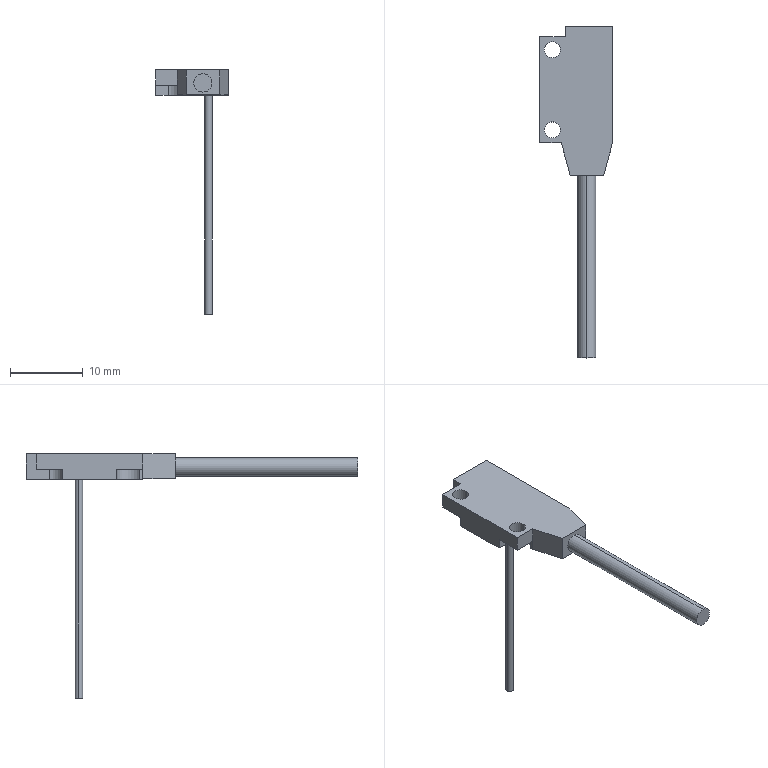Part | SolidWorks | features ICE 3, BaseBody 2 | 1 solid | 43 faces | box 10 x 45.5 x 33.5 mm | volume 726.533 mm3 | plane 31 | cylinder 12 | commonest cylinder face diameters 2.2 x4 1 x2 2 x2 2.5 x2 3.6 x2
STEP:
#1=CARTESIAN_POINT('',(-6.6,4.,21.4));
#2=VERTEX_POINT('',#1);
#3=CARTESIAN_POINT('',(-4.4,4.,21.4));
#4=VERTEX_POINT('',#3);
#5=CARTESIAN_POINT('',(-5.5,4.,21.4));
#6=DIRECTION('',(0.,0.,1.));
#7=DIRECTION('',(1.,0.,0.));
#8=AXIS2_PLACEMENT_3D('',#5,#6,#7);
#9=CIRCLE('',#8,1.1);
#10=EDGE_CURVE('',#2,#4,#9,.T.);
#11=ORIENTED_EDGE('',*,*,#10,.F.);
#12=CARTESIAN_POINT('',(-6.6,4.,23.5));
#13=VERTEX_POINT('',#12);
#14=CARTESIAN_POINT('',(-6.6,4.,20.));
#15=DIRECTION('',(0.,0.,1.));
#16=VECTOR('',#15,1000.);
#17=LINE('',#14,#16);
#18=EDGE_CURVE('',#2,#13,#17,.T.);
#19=ORIENTED_EDGE('',*,*,#18,.T.);
#20=CARTESIAN_POINT('',(-4.4,4.,23.5));
#21=VERTEX_POINT('',#20);
#22=CARTESIAN_POINT('',(-5.5,4.,23.5));
#23=DIRECTION('',(0.,0.,-1.));
#24=DIRECTION('',(1.,0.,0.));
#25=AXIS2_PLACEMENT_3D('',#22,#23,#24);
#26=CIRCLE('',#25,1.1);
#27=EDGE_CURVE('',#21,#13,#26,.T.);
#28=ORIENTED_EDGE('',*,*,#27,.F.);
#29=CARTESIAN_POINT('',(-4.4,4.,20.));
#30=DIRECTION('',(0.,0.,1.));
#31=VECTOR('',#30,1000.);
#32=LINE('',#29,#31);
#33=EDGE_CURVE('',#4,#21,#32,.T.);
#34=ORIENTED_EDGE('',*,*,#33,.F.);
#35=EDGE_LOOP('',(#11,#19,#28,#34));
#36=FACE_OUTER_BOUND('',#35,.T.);
#37=CARTESIAN_POINT('',(-5.5,4.,20.));
#38=DIRECTION('',(0.,0.,1.));
#39=DIRECTION('',(1.,0.,0.));
#40=AXIS2_PLACEMENT_3D('',#37,#38,#39);
#41=CYLINDRICAL_SURFACE('',#40,1.1);
#42=ADVANCED_FACE('',(#36),#41,.F.);
#43=CARTESIAN_POINT('',(-6.6,-7.,21.4));
#44=VERTEX_POINT('',#43);
#45=CARTESIAN_POINT('',(-4.4,-7.,21.4));
#46=VERTEX_POINT('',#45);
#47=CARTESIAN_POINT('',(-5.5,-7.,21.4));
#48=DIRECTION('',(0.,0.,1.));
#49=DIRECTION('',(1.,0.,0.));
#50=AXIS2_PLACEMENT_3D('',#47,#48,#49);
#51=CIRCLE('',#50,1.1);
#52=EDGE_CURVE('',#44,#46,#51,.T.);
#53=ORIENTED_EDGE('',*,*,#52,.F.);
#54=CARTESIAN_POINT('',(-6.6,-7.,23.5));
#55=VERTEX_POINT('',#54);
#56=CARTESIAN_POINT('',(-6.6,-7.,20.));
#57=DIRECTION('',(0.,0.,1.));
#58=VECTOR('',#57,1000.);
#59=LINE('',#56,#58);
#60=EDGE_CURVE('',#44,#55,#59,.T.);
#61=ORIENTED_EDGE('',*,*,#60,.T.);
#62=CARTESIAN_POINT('',(-4.4,-7.,23.5));
#63=VERTEX_POINT('',#62);
#64=CARTESIAN_POINT('',(-5.5,-7.,23.5));
#65=DIRECTION('',(0.,0.,-1.));
#66=DIRECTION('',(1.,0.,0.));
#67=AXIS2_PLACEMENT_3D('',#64,#65,#66);
#68=CIRCLE('',#67,1.1);
#69=EDGE_CURVE('',#63,#55,#68,.T.);
#70=ORIENTED_EDGE('',*,*,#69,.F.);
#71=CARTESIAN_POINT('',(-4.4,-7.,20.));
#72=DIRECTION('',(0.,0.,1.));
#73=VECTOR('',#72,1000.);
#74=LINE('',#71,#73);
#75=EDGE_CURVE('',#46,#63,#74,.T.);
#76=ORIENTED_EDGE('',*,*,#75,.F.);
#77=EDGE_LOOP('',(#53,#61,#70,#76));
#78=FACE_OUTER_BOUND('',#77,.T.);
#79=CARTESIAN_POINT('',(-5.5,-7.,20.));
#80=DIRECTION('',(0.,0.,1.));
#81=DIRECTION('',(1.,0.,0.));
#82=AXIS2_PLACEMENT_3D('',#79,#80,#81);
#83=CYLINDRICAL_SURFACE('',#82,1.1);
#84=ADVANCED_FACE('',(#78),#83,.F.);
#85=CARTESIAN_POINT('',(-0.75,-38.25,22.95));
#86=VERTEX_POINT('',#85);
#87=CARTESIAN_POINT('',(-0.75,-38.25,20.45));
#88=VERTEX_POINT('',#87);
#89=CARTESIAN_POINT('',(-0.75,-38.25,21.7));
#90=DIRECTION('',(0.,1.,0.));
#91=DIRECTION('',(0.,0.,1.));
#92=AXIS2_PLACEMENT_3D('',#89,#90,#91);
#93=CIRCLE('',#92,1.25);
#94=EDGE_CURVE('',#86,#88,#93,.T.);
#95=ORIENTED_EDGE('',*,*,#94,.T.);
#96=CARTESIAN_POINT('',(-0.75,-13.25,20.45));
#97=VERTEX_POINT('',#96);
#98=CARTESIAN_POINT('',(-0.75,-38.25,20.45));
#99=DIRECTION('',(0.,1.,0.));
#100=VECTOR('',#99,1000.);
#101=LINE('',#98,#100);
#102=EDGE_CURVE('',#88,#97,#101,.T.);
#103=ORIENTED_EDGE('',*,*,#102,.T.);
#104=CARTESIAN_POINT('',(-0.75,-13.25,22.95));
#105=VERTEX_POINT('',#104);
#106=CARTESIAN_POINT('',(-0.75,-13.25,21.7));
#107=DIRECTION('',(0.,-1.,0.));
#108=DIRECTION('',(0.,0.,1.));
#109=AXIS2_PLACEMENT_3D('',#106,#107,#108);
#110=CIRCLE('',#109,1.25);
#111=EDGE_CURVE('',#97,#105,#110,.T.);
#112=ORIENTED_EDGE('',*,*,#111,.T.);
#113=CARTESIAN_POINT('',(-0.75,-38.25,22.95));
#114=DIRECTION('',(0.,1.,0.));
#115=VECTOR('',#114,1000.);
#116=LINE('',#113,#115);
#117=EDGE_CURVE('',#86,#105,#116,.T.);
#118=ORIENTED_EDGE('',*,*,#117,.F.);
#119=EDGE_LOOP('',(#95,#103,#112,#118));
#120=FACE_OUTER_BOUND('',#119,.T.);
#121=CARTESIAN_POINT('',(-0.75,-38.25,21.7));
#122=DIRECTION('',(0.,1.,0.));
#123=DIRECTION('',(0.,0.,1.));
#124=AXIS2_PLACEMENT_3D('',#121,#122,#123);
#125=CYLINDRICAL_SURFACE('',#124,1.25);
#126=ADVANCED_FACE('',(#120),#125,.T.);
#127=CARTESIAN_POINT('',(1.,0.,20.1));
#128=VERTEX_POINT('',#127);
#129=CARTESIAN_POINT('',(-1.,0.,20.1));
#130=VERTEX_POINT('',#129);
#131=CARTESIAN_POINT('',(0.,0.,20.1));
#132=DIRECTION('',(0.,0.,-1.));
#133=DIRECTION('',(-1.,0.,0.));
#134=AXIS2_PLACEMENT_3D('',#131,#132,#133);
#135=CIRCLE('',#134,1.);
#136=EDGE_CURVE('',#128,#130,#135,.T.);
#137=ORIENTED_EDGE('',*,*,#136,.F.);
#138=CARTESIAN_POINT('',(1.,0.,20.));
#139=VERTEX_POINT('',#138);
#140=CARTESIAN_POINT('',(1.,0.,20.1));
#141=DIRECTION('',(0.,0.,-1.));
#142=VECTOR('',#141,1000.);
#143=LINE('',#140,#142);
#144=EDGE_CURVE('',#128,#139,#143,.T.);
#145=ORIENTED_EDGE('',*,*,#144,.T.);
#146=CARTESIAN_POINT('',(-1.,0.,20.));
#147=VERTEX_POINT('',#146);
#148=CARTESIAN_POINT('',(0.,0.,20.));
#149=DIRECTION('',(0.,0.,-1.));
#150=DIRECTION('',(-1.,0.,0.));
#151=AXIS2_PLACEMENT_3D('',#148,#149,#150);
#152=CIRCLE('',#151,1.);
#153=EDGE_CURVE('',#139,#147,#152,.T.);
#154=ORIENTED_EDGE('',*,*,#153,.T.);
#155=CARTESIAN_POINT('',(-1.,0.,20.1));
#156=DIRECTION('',(0.,0.,-1.));
#157=VECTOR('',#156,1000.);
#158=LINE('',#155,#157);
#159=EDGE_CURVE('',#130,#147,#158,.T.);
#160=ORIENTED_EDGE('',*,*,#159,.F.);
#161=EDGE_LOOP('',(#137,#145,#154,#160));
#162=FACE_OUTER_BOUND('',#161,.T.);
#163=CARTESIAN_POINT('',(0.,0.,20.1));
#164=DIRECTION('',(0.,0.,-1.));
#165=DIRECTION('',(-1.,0.,0.));
#166=AXIS2_PLACEMENT_3D('',#163,#164,#165);
#167=CYLINDRICAL_SURFACE('',#166,1.);
#168=ADVANCED_FACE('',(#162),#167,.F.);
#169=CARTESIAN_POINT('',(-0.5,0.,-10.));
#170=VERTEX_POINT('',#169);
#171=CARTESIAN_POINT('',(0.5,0.,-10.));
#172=VERTEX_POINT('',#171);
#173=CARTESIAN_POINT('',(0.,0.,-10.));
#174=DIRECTION('',(0.,0.,-1.));
#175=DIRECTION('',(-1.,0.,0.));
#176=AXIS2_PLACEMENT_3D('',#173,#174,#175);
#177=CIRCLE('',#176,0.5);
#178=EDGE_CURVE('',#170,#172,#177,.T.);
#179=ORIENTED_EDGE('',*,*,#178,.F.);
#180=CARTESIAN_POINT('',(-0.5,0.,20.1));
#181=VERTEX_POINT('',#180);
#182=CARTESIAN_POINT('',(-0.5,0.,-21.514));
#183=DIRECTION('',(0.,0.,1.));
#184=VECTOR('',#183,1000.);
#185=LINE('',#182,#184);
#186=EDGE_CURVE('',#170,#181,#185,.T.);
#187=ORIENTED_EDGE('',*,*,#186,.T.);
#188=CARTESIAN_POINT('',(0.5,0.,20.1));
#189=VERTEX_POINT('',#188);
#190=CARTESIAN_POINT('',(0.,0.,20.1));
#191=DIRECTION('',(0.,0.,1.));
#192=DIRECTION('',(1.,0.,0.));
#193=AXIS2_PLACEMENT_3D('',#190,#191,#192);
#194=CIRCLE('',#193,0.5);
#195=EDGE_CURVE('',#189,#181,#194,.T.);
#196=ORIENTED_EDGE('',*,*,#195,.F.);
#197=CARTESIAN_POINT('',(0.5,0.,-21.514));
#198=DIRECTION('',(0.,0.,1.));
#199=VECTOR('',#198,1000.);
#200=LINE('',#197,#199);
#201=EDGE_CURVE('',#172,#189,#200,.T.);
#202=ORIENTED_EDGE('',*,*,#201,.F.);
#203=EDGE_LOOP('',(#179,#187,#196,#202));
#204=FACE_OUTER_BOUND('',#203,.T.);
#205=CARTESIAN_POINT('',(0.,0.,-21.514));
#206=DIRECTION('',(0.,0.,1.));
#207=DIRECTION('',(1.,0.,0.));
#208=AXIS2_PLACEMENT_3D('',#205,#206,#207);
#209=CYLINDRICAL_SURFACE('',#208,0.5);
#210=ADVANCED_FACE('',(#204),#209,.T.);
#211=ORIENTED_EDGE('',*,*,#186,.F.);
#212=CARTESIAN_POINT('',(0.,0.,-10.));
#213=DIRECTION('',(0.,0.,-1.));
#214=DIRECTION('',(-1.,0.,0.));
#215=AXIS2_PLACEMENT_3D('',#212,#213,#214);
#216=CIRCLE('',#215,0.5);
#217=EDGE_CURVE('',#172,#170,#216,.T.);
#218=ORIENTED_EDGE('',*,*,#217,.F.);
#219=ORIENTED_EDGE('',*,*,#201,.T.);
#220=CARTESIAN_POINT('',(0.,0.,20.1));
#221=DIRECTION('',(0.,0.,1.));
#222=DIRECTION('',(1.,0.,0.));
#223=AXIS2_PLACEMENT_3D('',#220,#221,#222);
#224=CIRCLE('',#223,0.5);
#225=EDGE_CURVE('',#181,#189,#224,.T.);
#226=ORIENTED_EDGE('',*,*,#225,.F.);
#227=EDGE_LOOP('',(#211,#218,#219,#226));
#228=FACE_OUTER_BOUND('',#227,.T.);
#229=CARTESIAN_POINT('',(0.,0.,-21.514));
#230=DIRECTION('',(0.,0.,1.));
#231=DIRECTION('',(1.,0.,0.));
#232=AXIS2_PLACEMENT_3D('',#229,#230,#231);
#233=CYLINDRICAL_SURFACE('',#232,0.5);
#234=ADVANCED_FACE('',(#228),#233,.T.);
#235=CARTESIAN_POINT('',(0.,0.,20.1));
#236=DIRECTION('',(0.,0.,-1.));
#237=DIRECTION('',(-1.,0.,0.));
#238=AXIS2_PLACEMENT_3D('',#235,#236,#237);
#239=CIRCLE('',#238,1.);
#240=EDGE_CURVE('',#130,#128,#239,.T.);
#241=ORIENTED_EDGE('',*,*,#240,.T.);
#242=ORIENTED_EDGE('',*,*,#136,.T.);
#243=EDGE_LOOP('',(#241,#242));
#244=FACE_OUTER_BOUND('',#243,.T.);
#245=ORIENTED_EDGE('',*,*,#195,.T.);
#246=ORIENTED_EDGE('',*,*,#225,.T.);
#247=EDGE_LOOP('',(#245,#246));
#248=FACE_BOUND('',#247,.T.);
#249=CARTESIAN_POINT('',(0.,0.,20.1));
#250=DIRECTION('',(0.,0.,1.));
#251=DIRECTION('',(1.,0.,0.));
#252=AXIS2_PLACEMENT_3D('',#249,#250,#251);
#253=PLANE('',#252);
#254=ADVANCED_FACE('',(#244,#248),#253,.F.);
#255=ORIENTED_EDGE('',*,*,#27,.T.);
#256=CARTESIAN_POINT('',(-5.5,4.,23.5));
#257=DIRECTION('',(0.,0.,-1.));
#258=DIRECTION('',(1.,0.,0.));
#259=AXIS2_PLACEMENT_3D('',#256,#257,#258);
#260=CIRCLE('',#259,1.1);
#261=EDGE_CURVE('',#13,#21,#260,.T.);
#262=ORIENTED_EDGE('',*,*,#261,.T.);
#263=EDGE_LOOP('',(#255,#262));
#264=FACE_BOUND('',#263,.T.);
#265=ORIENTED_EDGE('',*,*,#69,.T.);
#266=CARTESIAN_POINT('',(-5.5,-7.,23.5));
#267=DIRECTION('',(0.,0.,-1.));
#268=DIRECTION('',(1.,0.,0.));
#269=AXIS2_PLACEMENT_3D('',#266,#267,#268);
#270=CIRCLE('',#269,1.1);
#271=EDGE_CURVE('',#55,#63,#270,.T.);
#272=ORIENTED_EDGE('',*,*,#271,.T.);
#273=EDGE_LOOP('',(#265,#272));
#274=FACE_BOUND('',#273,.T.);
#275=CARTESIAN_POINT('',(2.75,-8.75,23.5));
#276=VERTEX_POINT('',#275);
#277=CARTESIAN_POINT('',(2.75,7.25,23.5));
#278=VERTEX_POINT('',#277);
#279=CARTESIAN_POINT('',(2.75,-8.75,23.5));
#280=DIRECTION('',(0.,1.,0.));
#281=VECTOR('',#280,1000.);
#282=LINE('',#279,#281);
#283=EDGE_CURVE('',#276,#278,#282,.T.);
#284=ORIENTED_EDGE('',*,*,#283,.T.);
#285=CARTESIAN_POINT('',(-3.7,7.25,23.5));
#286=VERTEX_POINT('',#285);
#287=CARTESIAN_POINT('',(-7.25,7.25,23.5));
#288=DIRECTION('',(-1.,0.,0.));
#289=VECTOR('',#288,1000.);
#290=LINE('',#287,#289);
#291=EDGE_CURVE('',#278,#286,#290,.T.);
#292=ORIENTED_EDGE('',*,*,#291,.T.);
#293=CARTESIAN_POINT('',(-3.7,5.75,23.5));
#294=VERTEX_POINT('',#293);
#295=CARTESIAN_POINT('',(-3.7,7.25,23.5));
#296=DIRECTION('',(0.,1.,0.));
#297=VECTOR('',#296,1000.);
#298=LINE('',#295,#297);
#299=EDGE_CURVE('',#294,#286,#298,.T.);
#300=ORIENTED_EDGE('',*,*,#299,.F.);
#301=CARTESIAN_POINT('',(-7.25,5.75,23.5));
#302=VERTEX_POINT('',#301);
#303=CARTESIAN_POINT('',(-7.25,5.75,23.5));
#304=DIRECTION('',(-1.,0.,0.));
#305=VECTOR('',#304,1000.);
#306=LINE('',#303,#305);
#307=EDGE_CURVE('',#294,#302,#306,.T.);
#308=ORIENTED_EDGE('',*,*,#307,.T.);
#309=CARTESIAN_POINT('',(-7.25,-8.75,23.5));
#310=VERTEX_POINT('',#309);
#311=CARTESIAN_POINT('',(-7.25,-8.75,23.5));
#312=DIRECTION('',(0.,-1.,0.));
#313=VECTOR('',#312,1000.);
#314=LINE('',#311,#313);
#315=EDGE_CURVE('',#302,#310,#314,.T.);
#316=ORIENTED_EDGE('',*,*,#315,.T.);
#317=CARTESIAN_POINT('',(-4.25,-8.75,23.5));
#318=VERTEX_POINT('',#317);
#319=CARTESIAN_POINT('',(-7.25,-8.75,23.5));
#320=DIRECTION('',(1.,0.,0.));
#321=VECTOR('',#320,1000.);
#322=LINE('',#319,#321);
#323=EDGE_CURVE('',#310,#318,#322,.T.);
#324=ORIENTED_EDGE('',*,*,#323,.T.);
#325=CARTESIAN_POINT('',(-3.044,-13.25,23.5));
#326=VERTEX_POINT('',#325);
#327=CARTESIAN_POINT('',(-4.25,-8.75,23.5));
#328=DIRECTION('',(0.2588,-0.9659,0.));
#329=VECTOR('',#328,1000.);
#330=LINE('',#327,#329);
#331=EDGE_CURVE('',#318,#326,#330,.T.);
#332=ORIENTED_EDGE('',*,*,#331,.T.);
#333=CARTESIAN_POINT('',(1.544,-13.25,23.5));
#334=VERTEX_POINT('',#333);
#335=CARTESIAN_POINT('',(-7.25,-13.25,23.5));
#336=DIRECTION('',(1.,0.,0.));
#337=VECTOR('',#336,1000.);
#338=LINE('',#335,#337);
#339=EDGE_CURVE('',#326,#334,#338,.T.);
#340=ORIENTED_EDGE('',*,*,#339,.T.);
#341=CARTESIAN_POINT('',(1.544,-13.25,23.5));
#342=DIRECTION('',(0.2588,0.9659,0.));
#343=VECTOR('',#342,1000.);
#344=LINE('',#341,#343);
#345=EDGE_CURVE('',#334,#276,#344,.T.);
#346=ORIENTED_EDGE('',*,*,#345,.T.);
#347=EDGE_LOOP('',(#284,#292,#300,#308,#316,#324,#332,#340,#346));
#348=FACE_OUTER_BOUND('',#347,.T.);
#349=CARTESIAN_POINT('',(-7.25,-8.75,23.5));
#350=DIRECTION('',(0.,0.,1.));
#351=DIRECTION('',(1.,0.,0.));
#352=AXIS2_PLACEMENT_3D('',#349,#350,#351);
#353=PLANE('',#352);
#354=ADVANCED_FACE('',(#264,#274,#348),#353,.T.);
#355=ORIENTED_EDGE('',*,*,#18,.F.);
#356=CARTESIAN_POINT('',(-5.5,4.,21.4));
#357=DIRECTION('',(0.,0.,1.));
#358=DIRECTION('',(1.,0.,0.));
#359=AXIS2_PLACEMENT_3D('',#356,#357,#358);
#360=CIRCLE('',#359,1.1);
#361=EDGE_CURVE('',#4,#2,#360,.T.);
#362=ORIENTED_EDGE('',*,*,#361,.F.);
#363=ORIENTED_EDGE('',*,*,#33,.T.);
#364=ORIENTED_EDGE('',*,*,#261,.F.);
#365=EDGE_LOOP('',(#355,#362,#363,#364));
#366=FACE_OUTER_BOUND('',#365,.T.);
#367=CARTESIAN_POINT('',(-5.5,4.,20.));
#368=DIRECTION('',(0.,0.,1.));
#369=DIRECTION('',(1.,0.,0.));
#370=AXIS2_PLACEMENT_3D('',#367,#368,#369);
#371=CYLINDRICAL_SURFACE('',#370,1.1);
#372=ADVANCED_FACE('',(#366),#371,.F.);
#373=ORIENTED_EDGE('',*,*,#60,.F.);
#374=CARTESIAN_POINT('',(-5.5,-7.,21.4));
#375=DIRECTION('',(0.,0.,1.));
#376=DIRECTION('',(1.,0.,0.));
#377=AXIS2_PLACEMENT_3D('',#374,#375,#376);
#378=CIRCLE('',#377,1.1);
#379=EDGE_CURVE('',#46,#44,#378,.T.);
#380=ORIENTED_EDGE('',*,*,#379,.F.);
#381=ORIENTED_EDGE('',*,*,#75,.T.);
#382=ORIENTED_EDGE('',*,*,#271,.F.);
#383=EDGE_LOOP('',(#373,#380,#381,#382));
#384=FACE_OUTER_BOUND('',#383,.T.);
#385=CARTESIAN_POINT('',(-5.5,-7.,20.));
#386=DIRECTION('',(0.,0.,1.));
#387=DIRECTION('',(1.,0.,0.));
#388=AXIS2_PLACEMENT_3D('',#385,#386,#387);
#389=CYLINDRICAL_SURFACE('',#388,1.1);
#390=ADVANCED_FACE('',(#384),#389,.F.);
#391=ORIENTED_EDGE('',*,*,#291,.F.);
#392=CARTESIAN_POINT('',(2.75,7.25,20.));
#393=VERTEX_POINT('',#392);
#394=CARTESIAN_POINT('',(2.75,7.25,23.5));
#395=DIRECTION('',(0.,0.,1.));
#396=VECTOR('',#395,1000.);
#397=LINE('',#394,#396);
#398=EDGE_CURVE('',#393,#278,#397,.T.);
#399=ORIENTED_EDGE('',*,*,#398,.F.);
#400=CARTESIAN_POINT('',(-3.7,7.25,20.));
#401=VERTEX_POINT('',#400);
#402=CARTESIAN_POINT('',(-7.25,7.25,20.));
#403=DIRECTION('',(1.,0.,0.));
#404=VECTOR('',#403,1000.);
#405=LINE('',#402,#404);
#406=EDGE_CURVE('',#401,#393,#405,.T.);
#407=ORIENTED_EDGE('',*,*,#406,.F.);
#408=CARTESIAN_POINT('',(-3.7,7.25,23.5));
#409=DIRECTION('',(0.,0.,-1.));
#410=VECTOR('',#409,1000.);
#411=LINE('',#408,#410);
#412=EDGE_CURVE('',#286,#401,#411,.T.);
#413=ORIENTED_EDGE('',*,*,#412,.F.);
#414=EDGE_LOOP('',(#391,#399,#407,#413));
#415=FACE_OUTER_BOUND('',#414,.T.);
#416=CARTESIAN_POINT('',(-7.25,7.25,23.5));
#417=DIRECTION('',(0.,-1.,0.));
#418=DIRECTION('',(0.,0.,-1.));
#419=AXIS2_PLACEMENT_3D('',#416,#417,#418);
#420=PLANE('',#419);
#421=ADVANCED_FACE('',(#415),#420,.F.);
#422=ORIENTED_EDGE('',*,*,#398,.T.);
#423=ORIENTED_EDGE('',*,*,#283,.F.);
#424=CARTESIAN_POINT('',(2.75,-8.75,20.1));
#425=VERTEX_POINT('',#424);
#426=CARTESIAN_POINT('',(2.75,-8.75,23.5));
#427=DIRECTION('',(0.,0.,1.));
#428=VECTOR('',#427,1000.);
#429=LINE('',#426,#428);
#430=EDGE_CURVE('',#425,#276,#429,.T.);
#431=ORIENTED_EDGE('',*,*,#430,.F.);
#432=CARTESIAN_POINT('',(2.75,-8.75,20.));
#433=VERTEX_POINT('',#432);
#434=CARTESIAN_POINT('',(2.75,-8.75,20.1));
#435=DIRECTION('',(0.,0.,1.));
#436=VECTOR('',#435,1000.);
#437=LINE('',#434,#436);
#438=EDGE_CURVE('',#433,#425,#437,.T.);
#439=ORIENTED_EDGE('',*,*,#438,.F.);
#440=CARTESIAN_POINT('',(2.75,7.25,20.));
#441=DIRECTION('',(0.,-1.,0.));
#442=VECTOR('',#441,1000.);
#443=LINE('',#440,#442);
#444=EDGE_CURVE('',#393,#433,#443,.T.);
#445=ORIENTED_EDGE('',*,*,#444,.F.);
#446=EDGE_LOOP('',(#422,#423,#431,#439,#445));
#447=FACE_OUTER_BOUND('',#446,.T.);
#448=CARTESIAN_POINT('',(2.75,7.25,23.5));
#449=DIRECTION('',(-1.,0.,0.));
#450=DIRECTION('',(0.,-1.,0.));
#451=AXIS2_PLACEMENT_3D('',#448,#449,#450);
#452=PLANE('',#451);
#453=ADVANCED_FACE('',(#447),#452,.F.);
#454=ORIENTED_EDGE('',*,*,#430,.T.);
#455=ORIENTED_EDGE('',*,*,#345,.F.);
#456=CARTESIAN_POINT('',(1.544,-13.25,20.1));
#457=VERTEX_POINT('',#456);
#458=CARTESIAN_POINT('',(1.544,-13.25,23.5));
#459=DIRECTION('',(0.,0.,1.));
#460=VECTOR('',#459,1000.);
#461=LINE('',#458,#460);
#462=EDGE_CURVE('',#457,#334,#461,.T.);
#463=ORIENTED_EDGE('',*,*,#462,.F.);
#464=CARTESIAN_POINT('',(2.75,-8.75,20.1));
#465=DIRECTION('',(-0.2588,-0.9659,0.));
#466=VECTOR('',#465,1000.);
#467=LINE('',#464,#466);
#468=EDGE_CURVE('',#425,#457,#467,.T.);
#469=ORIENTED_EDGE('',*,*,#468,.F.);
#470=EDGE_LOOP('',(#454,#455,#463,#469));
#471=FACE_OUTER_BOUND('',#470,.T.);
#472=CARTESIAN_POINT('',(2.75,-8.75,23.5));
#473=DIRECTION('',(-0.9659,0.2588,0.));
#474=DIRECTION('',(-0.2588,-0.9659,0.));
#475=AXIS2_PLACEMENT_3D('',#472,#473,#474);
#476=PLANE('',#475);
#477=ADVANCED_FACE('',(#471),#476,.F.);
#478=ORIENTED_EDGE('',*,*,#462,.T.);
#479=ORIENTED_EDGE('',*,*,#339,.F.);
#480=CARTESIAN_POINT('',(-3.044,-13.25,20.1));
#481=VERTEX_POINT('',#480);
#482=CARTESIAN_POINT('',(-3.044,-13.25,23.5));
#483=DIRECTION('',(0.,0.,1.));
#484=VECTOR('',#483,1000.);
#485=LINE('',#482,#484);
#486=EDGE_CURVE('',#481,#326,#485,.T.);
#487=ORIENTED_EDGE('',*,*,#486,.F.);
#488=CARTESIAN_POINT('',(1.544,-13.25,20.1));
#489=DIRECTION('',(-1.,0.,0.));
#490=VECTOR('',#489,1000.);
#491=LINE('',#488,#490);
#492=EDGE_CURVE('',#457,#481,#491,.T.);
#493=ORIENTED_EDGE('',*,*,#492,.F.);
#494=EDGE_LOOP('',(#478,#479,#487,#493));
#495=FACE_OUTER_BOUND('',#494,.T.);
#496=CARTESIAN_POINT('',(-0.75,-13.25,21.7));
#497=DIRECTION('',(0.,-1.,0.));
#498=DIRECTION('',(0.,0.,1.));
#499=AXIS2_PLACEMENT_3D('',#496,#497,#498);
#500=CIRCLE('',#499,1.25);
#501=EDGE_CURVE('',#105,#97,#500,.T.);
#502=ORIENTED_EDGE('',*,*,#501,.F.);
#503=ORIENTED_EDGE('',*,*,#111,.F.);
#504=EDGE_LOOP('',(#502,#503));
#505=FACE_BOUND('',#504,.T.);
#506=CARTESIAN_POINT('',(1.544,-13.25,23.5));
#507=DIRECTION('',(0.,1.,0.));
#508=DIRECTION('',(0.,0.,1.));
#509=AXIS2_PLACEMENT_3D('',#506,#507,#508);
#510=PLANE('',#509);
#511=ADVANCED_FACE('',(#495,#505),#510,.F.);
#512=ORIENTED_EDGE('',*,*,#486,.T.);
#513=ORIENTED_EDGE('',*,*,#331,.F.);
#514=CARTESIAN_POINT('',(-4.25,-8.75,21.4));
#515=VERTEX_POINT('',#514);
#516=CARTESIAN_POINT('',(-4.25,-8.75,23.5));
#517=DIRECTION('',(0.,0.,1.));
#518=VECTOR('',#517,1000.);
#519=LINE('',#516,#518);
#520=EDGE_CURVE('',#515,#318,#519,.T.);
#521=ORIENTED_EDGE('',*,*,#520,.F.);
#522=CARTESIAN_POINT('',(-4.25,-8.75,20.1));
#523=VERTEX_POINT('',#522);
#524=CARTESIAN_POINT('',(-4.25,-8.75,23.5));
#525=DIRECTION('',(0.,0.,1.));
#526=VECTOR('',#525,1000.);
#527=LINE('',#524,#526);
#528=EDGE_CURVE('',#523,#515,#527,.T.);
#529=ORIENTED_EDGE('',*,*,#528,.F.);
#530=CARTESIAN_POINT('',(-3.044,-13.25,20.1));
#531=DIRECTION('',(-0.2588,0.9659,0.));
#532=VECTOR('',#531,1000.);
#533=LINE('',#530,#532);
#534=EDGE_CURVE('',#481,#523,#533,.T.);
#535=ORIENTED_EDGE('',*,*,#534,.F.);
#536=EDGE_LOOP('',(#512,#513,#521,#529,#535));
#537=FACE_OUTER_BOUND('',#536,.T.);
#538=CARTESIAN_POINT('',(-3.044,-13.25,23.5));
#539=DIRECTION('',(0.9659,0.2588,0.));
#540=DIRECTION('',(-0.2588,0.9659,0.));
#541=AXIS2_PLACEMENT_3D('',#538,#539,#540);
#542=PLANE('',#541);
#543=ADVANCED_FACE('',(#537),#542,.F.);
#544=CARTESIAN_POINT('',(-7.25,-8.75,21.4));
#545=VERTEX_POINT('',#544);
#546=CARTESIAN_POINT('',(-7.25,-8.75,21.4));
#547=DIRECTION('',(-1.,0.,0.));
#548=VECTOR('',#547,1000.);
#549=LINE('',#546,#548);
#550=EDGE_CURVE('',#515,#545,#549,.T.);
#551=ORIENTED_EDGE('',*,*,#550,.F.);
#552=ORIENTED_EDGE('',*,*,#520,.T.);
#553=ORIENTED_EDGE('',*,*,#323,.F.);
#554=CARTESIAN_POINT('',(-7.25,-8.75,23.5));
#555=DIRECTION('',(0.,0.,1.));
#556=VECTOR('',#555,1000.);
#557=LINE('',#554,#556);
#558=EDGE_CURVE('',#545,#310,#557,.T.);
#559=ORIENTED_EDGE('',*,*,#558,.F.);
#560=EDGE_LOOP('',(#551,#552,#553,#559));
#561=FACE_OUTER_BOUND('',#560,.T.);
#562=CARTESIAN_POINT('',(-7.25,-8.75,23.5));
#563=DIRECTION('',(0.,1.,0.));
#564=DIRECTION('',(0.,0.,1.));
#565=AXIS2_PLACEMENT_3D('',#562,#563,#564);
#566=PLANE('',#565);
#567=ADVANCED_FACE('',(#561),#566,.F.);
#568=CARTESIAN_POINT('',(-7.25,5.75,21.4));
#569=VERTEX_POINT('',#568);
#570=CARTESIAN_POINT('',(-7.25,5.75,23.5));
#571=DIRECTION('',(0.,0.,1.));
#572=VECTOR('',#571,1000.);
#573=LINE('',#570,#572);
#574=EDGE_CURVE('',#569,#302,#573,.T.);
#575=ORIENTED_EDGE('',*,*,#574,.F.);
#576=CARTESIAN_POINT('',(-7.25,2.2,21.4));
#577=VERTEX_POINT('',#576);
#578=CARTESIAN_POINT('',(-7.25,7.25,21.4));
#579=DIRECTION('',(0.,1.,0.));
#580=VECTOR('',#579,1000.);
#581=LINE('',#578,#580);
#582=EDGE_CURVE('',#577,#569,#581,.T.);
#583=ORIENTED_EDGE('',*,*,#582,.F.);
#584=CARTESIAN_POINT('',(-7.25,2.2,20.));
#585=VERTEX_POINT('',#584);
#586=CARTESIAN_POINT('',(-7.25,2.2,21.4));
#587=DIRECTION('',(0.,0.,1.));
#588=VECTOR('',#587,1000.);
#589=LINE('',#586,#588);
#590=EDGE_CURVE('',#585,#577,#589,.T.);
#591=ORIENTED_EDGE('',*,*,#590,.F.);
#592=CARTESIAN_POINT('',(-7.25,-5.2,20.));
#593=VERTEX_POINT('',#592);
#594=CARTESIAN_POINT('',(-7.25,7.25,20.));
#595=DIRECTION('',(0.,1.,0.));
#596=VECTOR('',#595,1000.);
#597=LINE('',#594,#596);
#598=EDGE_CURVE('',#593,#585,#597,.T.);
#599=ORIENTED_EDGE('',*,*,#598,.F.);
#600=CARTESIAN_POINT('',(-7.25,-5.2,21.4));
#601=VERTEX_POINT('',#600);
#602=CARTESIAN_POINT('',(-7.25,-5.2,21.4));
#603=DIRECTION('',(0.,0.,-1.));
#604=VECTOR('',#603,1000.);
#605=LINE('',#602,#604);
#606=EDGE_CURVE('',#601,#593,#605,.T.);
#607=ORIENTED_EDGE('',*,*,#606,.F.);
#608=CARTESIAN_POINT('',(-7.25,7.25,21.4));
#609=DIRECTION('',(0.,1.,0.));
#610=VECTOR('',#609,1000.);
#611=LINE('',#608,#610);
#612=EDGE_CURVE('',#545,#601,#611,.T.);
#613=ORIENTED_EDGE('',*,*,#612,.F.);
#614=ORIENTED_EDGE('',*,*,#558,.T.);
#615=ORIENTED_EDGE('',*,*,#315,.F.);
#616=EDGE_LOOP('',(#575,#583,#591,#599,#607,#613,#614,#615));
#617=FACE_OUTER_BOUND('',#616,.T.);
#618=CARTESIAN_POINT('',(-7.25,7.25,23.5));
#619=DIRECTION('',(1.,0.,0.));
#620=DIRECTION('',(0.,1.,0.));
#621=AXIS2_PLACEMENT_3D('',#618,#619,#620);
#622=PLANE('',#621);
#623=ADVANCED_FACE('',(#617),#622,.F.);
#624=CARTESIAN_POINT('',(-3.7,5.75,21.4));
#625=VERTEX_POINT('',#624);
#626=CARTESIAN_POINT('',(-3.7,5.75,20.));
#627=DIRECTION('',(0.,0.,1.));
#628=VECTOR('',#627,1000.);
#629=LINE('',#626,#628);
#630=EDGE_CURVE('',#625,#294,#629,.T.);
#631=ORIENTED_EDGE('',*,*,#630,.F.);
#632=CARTESIAN_POINT('',(-7.7,5.75,21.4));
#633=DIRECTION('',(1.,0.,0.));
#634=VECTOR('',#633,1000.);
#635=LINE('',#632,#634);
#636=EDGE_CURVE('',#569,#625,#635,.T.);
#637=ORIENTED_EDGE('',*,*,#636,.F.);
#638=ORIENTED_EDGE('',*,*,#574,.T.);
#639=ORIENTED_EDGE('',*,*,#307,.F.);
#640=EDGE_LOOP('',(#631,#637,#638,#639));
#641=FACE_OUTER_BOUND('',#640,.T.);
#642=CARTESIAN_POINT('',(-7.7,5.75,20.));
#643=DIRECTION('',(0.,-1.,0.));
#644=DIRECTION('',(0.,0.,-1.));
#645=AXIS2_PLACEMENT_3D('',#642,#643,#644);
#646=PLANE('',#645);
#647=ADVANCED_FACE('',(#641),#646,.F.);
#648=ORIENTED_EDGE('',*,*,#361,.T.);
#649=ORIENTED_EDGE('',*,*,#10,.T.);
#650=EDGE_LOOP('',(#648,#649));
#651=FACE_BOUND('',#650,.T.);
#652=ORIENTED_EDGE('',*,*,#636,.T.);
#653=CARTESIAN_POINT('',(-3.7,4.,21.4));
#654=VERTEX_POINT('',#653);
#655=CARTESIAN_POINT('',(-3.7,4.,21.4));
#656=DIRECTION('',(0.,1.,0.));
#657=VECTOR('',#656,1000.);
#658=LINE('',#655,#657);
#659=EDGE_CURVE('',#654,#625,#658,.T.);
#660=ORIENTED_EDGE('',*,*,#659,.F.);
#661=CARTESIAN_POINT('',(-5.5,2.2,21.4));
#662=VERTEX_POINT('',#661);
#663=CARTESIAN_POINT('',(-5.5,4.,21.4));
#664=DIRECTION('',(0.,0.,1.));
#665=DIRECTION('',(-1.,0.,0.));
#666=AXIS2_PLACEMENT_3D('',#663,#664,#665);
#667=CIRCLE('',#666,1.8);
#668=EDGE_CURVE('',#662,#654,#667,.T.);
#669=ORIENTED_EDGE('',*,*,#668,.F.);
#670=CARTESIAN_POINT('',(-5.5,2.2,21.4));
#671=DIRECTION('',(1.,0.,0.));
#672=VECTOR('',#671,1000.);
#673=LINE('',#670,#672);
#674=EDGE_CURVE('',#577,#662,#673,.T.);
#675=ORIENTED_EDGE('',*,*,#674,.F.);
#676=ORIENTED_EDGE('',*,*,#582,.T.);
#677=EDGE_LOOP('',(#652,#660,#669,#675,#676));
#678=FACE_OUTER_BOUND('',#677,.T.);
#679=CARTESIAN_POINT('',(-5.5,4.,21.4));
#680=DIRECTION('',(0.,0.,1.));
#681=DIRECTION('',(1.,0.,0.));
#682=AXIS2_PLACEMENT_3D('',#679,#680,#681);
#683=PLANE('',#682);
#684=ADVANCED_FACE('',(#651,#678),#683,.F.);
#685=ORIENTED_EDGE('',*,*,#379,.T.);
#686=ORIENTED_EDGE('',*,*,#52,.T.);
#687=EDGE_LOOP('',(#685,#686));
#688=FACE_BOUND('',#687,.T.);
#689=CARTESIAN_POINT('',(-4.25,-8.295,21.4));
#690=VERTEX_POINT('',#689);
#691=CARTESIAN_POINT('',(-4.25,-7.,21.4));
#692=DIRECTION('',(0.,1.,0.));
#693=VECTOR('',#692,1000.);
#694=LINE('',#691,#693);
#695=EDGE_CURVE('',#515,#690,#694,.T.);
#696=ORIENTED_EDGE('',*,*,#695,.F.);
#697=ORIENTED_EDGE('',*,*,#550,.T.);
#698=ORIENTED_EDGE('',*,*,#612,.T.);
#699=CARTESIAN_POINT('',(-5.5,-5.2,21.4));
#700=VERTEX_POINT('',#699);
#701=CARTESIAN_POINT('',(-5.5,-5.2,21.4));
#702=DIRECTION('',(-1.,0.,0.));
#703=VECTOR('',#702,1000.);
#704=LINE('',#701,#703);
#705=EDGE_CURVE('',#700,#601,#704,.T.);
#706=ORIENTED_EDGE('',*,*,#705,.F.);
#707=CARTESIAN_POINT('',(-5.5,-7.,21.4));
#708=DIRECTION('',(0.,0.,1.));
#709=DIRECTION('',(-1.,0.,0.));
#710=AXIS2_PLACEMENT_3D('',#707,#708,#709);
#711=CIRCLE('',#710,1.8);
#712=EDGE_CURVE('',#690,#700,#711,.T.);
#713=ORIENTED_EDGE('',*,*,#712,.F.);
#714=EDGE_LOOP('',(#696,#697,#698,#706,#713));
#715=FACE_OUTER_BOUND('',#714,.T.);
#716=CARTESIAN_POINT('',(-5.5,-7.,21.4));
#717=DIRECTION('',(0.,0.,1.));
#718=DIRECTION('',(1.,0.,0.));
#719=AXIS2_PLACEMENT_3D('',#716,#717,#718);
#720=PLANE('',#719);
#721=ADVANCED_FACE('',(#688,#715),#720,.F.);
#722=CARTESIAN_POINT('',(-3.7,4.,20.));
#723=VERTEX_POINT('',#722);
#724=CARTESIAN_POINT('',(-3.7,7.25,20.));
#725=DIRECTION('',(0.,-1.,0.));
#726=VECTOR('',#725,1000.);
#727=LINE('',#724,#726);
#728=EDGE_CURVE('',#401,#723,#727,.T.);
#729=ORIENTED_EDGE('',*,*,#728,.T.);
#730=CARTESIAN_POINT('',(-3.7,4.,21.4));
#731=DIRECTION('',(0.,0.,1.));
#732=VECTOR('',#731,1000.);
#733=LINE('',#730,#732);
#734=EDGE_CURVE('',#723,#654,#733,.T.);
#735=ORIENTED_EDGE('',*,*,#734,.T.);
#736=ORIENTED_EDGE('',*,*,#659,.T.);
#737=ORIENTED_EDGE('',*,*,#630,.T.);
#738=ORIENTED_EDGE('',*,*,#299,.T.);
#739=ORIENTED_EDGE('',*,*,#412,.T.);
#740=EDGE_LOOP('',(#729,#735,#736,#737,#738,#739));
#741=FACE_OUTER_BOUND('',#740,.T.);
#742=CARTESIAN_POINT('',(-3.7,7.25,21.4));
#743=DIRECTION('',(-1.,0.,0.));
#744=DIRECTION('',(0.,-1.,0.));
#745=AXIS2_PLACEMENT_3D('',#742,#743,#744);
#746=PLANE('',#745);
#747=ADVANCED_FACE('',(#741),#746,.T.);
#748=CARTESIAN_POINT('',(-4.25,-8.295,20.));
#749=VERTEX_POINT('',#748);
#750=CARTESIAN_POINT('',(-4.25,-8.75,20.));
#751=VERTEX_POINT('',#750);
#752=CARTESIAN_POINT('',(-4.25,-8.75,20.));
#753=DIRECTION('',(0.,-1.,0.));
#754=VECTOR('',#753,1000.);
#755=LINE('',#752,#754);
#756=EDGE_CURVE('',#749,#751,#755,.T.);
#757=ORIENTED_EDGE('',*,*,#756,.F.);
#758=CARTESIAN_POINT('',(-5.5,-5.2,20.));
#759=VERTEX_POINT('',#758);
#760=CARTESIAN_POINT('',(-5.5,-7.,20.));
#761=DIRECTION('',(0.,0.,-1.));
#762=DIRECTION('',(-1.,0.,0.));
#763=AXIS2_PLACEMENT_3D('',#760,#761,#762);
#764=CIRCLE('',#763,1.8);
#765=EDGE_CURVE('',#759,#749,#764,.T.);
#766=ORIENTED_EDGE('',*,*,#765,.F.);
#767=CARTESIAN_POINT('',(-7.25,-5.2,20.));
#768=DIRECTION('',(1.,0.,0.));
#769=VECTOR('',#768,1000.);
#770=LINE('',#767,#769);
#771=EDGE_CURVE('',#593,#759,#770,.T.);
#772=ORIENTED_EDGE('',*,*,#771,.F.);
#773=ORIENTED_EDGE('',*,*,#598,.T.);
#774=CARTESIAN_POINT('',(-5.5,2.2,20.));
#775=VERTEX_POINT('',#774);
#776=CARTESIAN_POINT('',(-7.25,2.2,20.));
#777=DIRECTION('',(-1.,0.,0.));
#778=VECTOR('',#777,1000.);
#779=LINE('',#776,#778);
#780=EDGE_CURVE('',#775,#585,#779,.T.);
#781=ORIENTED_EDGE('',*,*,#780,.F.);
#782=CARTESIAN_POINT('',(-5.5,4.,20.));
#783=DIRECTION('',(0.,0.,-1.));
#784=DIRECTION('',(-1.,0.,0.));
#785=AXIS2_PLACEMENT_3D('',#782,#783,#784);
#786=CIRCLE('',#785,1.8);
#787=EDGE_CURVE('',#723,#775,#786,.T.);
#788=ORIENTED_EDGE('',*,*,#787,.F.);
#789=ORIENTED_EDGE('',*,*,#728,.F.);
#790=ORIENTED_EDGE('',*,*,#406,.T.);
#791=ORIENTED_EDGE('',*,*,#444,.T.);
#792=CARTESIAN_POINT('',(-7.25,-8.75,20.));
#793=DIRECTION('',(1.,0.,0.));
#794=VECTOR('',#793,1000.);
#795=LINE('',#792,#794);
#796=EDGE_CURVE('',#751,#433,#795,.T.);
#797=ORIENTED_EDGE('',*,*,#796,.F.);
#798=EDGE_LOOP('',(#757,#766,#772,#773,#781,#788,#789,#790,#791,#797));
#799=FACE_OUTER_BOUND('',#798,.T.);
#800=CARTESIAN_POINT('',(2.25,4.95,20.));
#801=VERTEX_POINT('',#800);
#802=CARTESIAN_POINT('',(0.05,4.95,20.));
#803=VERTEX_POINT('',#802);
#804=CARTESIAN_POINT('',(-7.25,4.95,20.));
#805=DIRECTION('',(-1.,0.,0.));
#806=VECTOR('',#805,1000.);
#807=LINE('',#804,#806);
#808=EDGE_CURVE('',#801,#803,#807,.T.);
#809=ORIENTED_EDGE('',*,*,#808,.F.);
#810=CARTESIAN_POINT('',(2.25,6.95,20.));
#811=VERTEX_POINT('',#810);
#812=CARTESIAN_POINT('',(2.25,-8.75,20.));
#813=DIRECTION('',(0.,-1.,0.));
#814=VECTOR('',#813,1000.);
#815=LINE('',#812,#814);
#816=EDGE_CURVE('',#811,#801,#815,.T.);
#817=ORIENTED_EDGE('',*,*,#816,.F.);
#818=CARTESIAN_POINT('',(0.05,6.95,20.));
#819=VERTEX_POINT('',#818);
#820=CARTESIAN_POINT('',(-7.25,6.95,20.));
#821=DIRECTION('',(1.,0.,0.));
#822=VECTOR('',#821,1000.);
#823=LINE('',#820,#822);
#824=EDGE_CURVE('',#819,#811,#823,.T.);
#825=ORIENTED_EDGE('',*,*,#824,.F.);
#826=CARTESIAN_POINT('',(0.05,-8.75,20.));
#827=DIRECTION('',(0.,1.,0.));
#828=VECTOR('',#827,1000.);
#829=LINE('',#826,#828);
#830=EDGE_CURVE('',#803,#819,#829,.T.);
#831=ORIENTED_EDGE('',*,*,#830,.F.);
#832=EDGE_LOOP('',(#809,#817,#825,#831));
#833=FACE_BOUND('',#832,.T.);
#834=CARTESIAN_POINT('',(0.,0.,20.));
#835=DIRECTION('',(0.,0.,-1.));
#836=DIRECTION('',(-1.,0.,0.));
#837=AXIS2_PLACEMENT_3D('',#834,#835,#836);
#838=CIRCLE('',#837,1.);
#839=EDGE_CURVE('',#147,#139,#838,.T.);
#840=ORIENTED_EDGE('',*,*,#839,.F.);
#841=ORIENTED_EDGE('',*,*,#153,.F.);
#842=EDGE_LOOP('',(#840,#841));
#843=FACE_BOUND('',#842,.T.);
#844=CARTESIAN_POINT('',(-0.75,4.95,20.));
#845=VERTEX_POINT('',#844);
#846=CARTESIAN_POINT('',(-2.95,4.95,20.));
#847=VERTEX_POINT('',#846);
#848=CARTESIAN_POINT('',(-7.25,4.95,20.));
#849=DIRECTION('',(-1.,0.,0.));
#850=VECTOR('',#849,1000.);
#851=LINE('',#848,#850);
#852=EDGE_CURVE('',#845,#847,#851,.T.);
#853=ORIENTED_EDGE('',*,*,#852,.F.);
#854=CARTESIAN_POINT('',(-0.75,6.95,20.));
#855=VERTEX_POINT('',#854);
#856=CARTESIAN_POINT('',(-0.75,-8.75,20.));
#857=DIRECTION('',(0.,-1.,0.));
#858=VECTOR('',#857,1000.);
#859=LINE('',#856,#858);
#860=EDGE_CURVE('',#855,#845,#859,.T.);
#861=ORIENTED_EDGE('',*,*,#860,.F.);
#862=CARTESIAN_POINT('',(-2.95,6.95,20.));
#863=VERTEX_POINT('',#862);
#864=CARTESIAN_POINT('',(-7.25,6.95,20.));
#865=DIRECTION('',(1.,0.,0.));
#866=VECTOR('',#865,1000.);
#867=LINE('',#864,#866);
#868=EDGE_CURVE('',#863,#855,#867,.T.);
#869=ORIENTED_EDGE('',*,*,#868,.F.);
#870=CARTESIAN_POINT('',(-2.95,-8.75,20.));
#871=DIRECTION('',(0.,1.,0.));
#872=VECTOR('',#871,1000.);
#873=LINE('',#870,#872);
#874=EDGE_CURVE('',#847,#863,#873,.T.);
#875=ORIENTED_EDGE('',*,*,#874,.F.);
#876=EDGE_LOOP('',(#853,#861,#869,#875));
#877=FACE_BOUND('',#876,.T.);
#878=CARTESIAN_POINT('',(-7.25,-8.75,20.));
#879=DIRECTION('',(0.,0.,1.));
#880=DIRECTION('',(1.,0.,0.));
#881=AXIS2_PLACEMENT_3D('',#878,#879,#880);
#882=PLANE('',#881);
#883=ADVANCED_FACE('',(#799,#833,#843,#877),#882,.F.);
#884=ORIENTED_EDGE('',*,*,#468,.T.);
#885=ORIENTED_EDGE('',*,*,#492,.T.);
#886=ORIENTED_EDGE('',*,*,#534,.T.);
#887=CARTESIAN_POINT('',(-4.25,-8.75,20.1));
#888=DIRECTION('',(1.,0.,0.));
#889=VECTOR('',#888,1000.);
#890=LINE('',#887,#889);
#891=EDGE_CURVE('',#523,#425,#890,.T.);
#892=ORIENTED_EDGE('',*,*,#891,.T.);
#893=EDGE_LOOP('',(#884,#885,#886,#892));
#894=FACE_OUTER_BOUND('',#893,.T.);
#895=CARTESIAN_POINT('',(-4.25,-8.75,20.1));
#896=DIRECTION('',(0.,0.,-1.));
#897=DIRECTION('',(-1.,0.,0.));
#898=AXIS2_PLACEMENT_3D('',#895,#896,#897);
#899=PLANE('',#898);
#900=ADVANCED_FACE('',(#894),#899,.T.);
#901=ORIENTED_EDGE('',*,*,#102,.F.);
#902=CARTESIAN_POINT('',(-0.75,-38.25,21.7));
#903=DIRECTION('',(0.,1.,0.));
#904=DIRECTION('',(0.,0.,1.));
#905=AXIS2_PLACEMENT_3D('',#902,#903,#904);
#906=CIRCLE('',#905,1.25);
#907=EDGE_CURVE('',#88,#86,#906,.T.);
#908=ORIENTED_EDGE('',*,*,#907,.T.);
#909=ORIENTED_EDGE('',*,*,#117,.T.);
#910=ORIENTED_EDGE('',*,*,#501,.T.);
#911=EDGE_LOOP('',(#901,#908,#909,#910));
#912=FACE_OUTER_BOUND('',#911,.T.);
#913=CARTESIAN_POINT('',(-0.75,-38.25,21.7));
#914=DIRECTION('',(0.,1.,0.));
#915=DIRECTION('',(0.,0.,1.));
#916=AXIS2_PLACEMENT_3D('',#913,#914,#915);
#917=CYLINDRICAL_SURFACE('',#916,1.25);
#918=ADVANCED_FACE('',(#912),#917,.T.);
#919=ORIENTED_EDGE('',*,*,#695,.T.);
#920=CARTESIAN_POINT('',(-4.25,-8.295,21.4));
#921=DIRECTION('',(0.,0.,-1.));
#922=VECTOR('',#921,1000.);
#923=LINE('',#920,#922);
#924=EDGE_CURVE('',#690,#749,#923,.T.);
#925=ORIENTED_EDGE('',*,*,#924,.T.);
#926=ORIENTED_EDGE('',*,*,#756,.T.);
#927=CARTESIAN_POINT('',(-4.25,-8.75,21.4));
#928=DIRECTION('',(0.,0.,1.));
#929=VECTOR('',#928,1000.);
#930=LINE('',#927,#929);
#931=EDGE_CURVE('',#751,#523,#930,.T.);
#932=ORIENTED_EDGE('',*,*,#931,.T.);
#933=ORIENTED_EDGE('',*,*,#528,.T.);
#934=EDGE_LOOP('',(#919,#925,#926,#932,#933));
#935=FACE_OUTER_BOUND('',#934,.T.);
#936=CARTESIAN_POINT('',(-4.25,-8.295,21.4));
#937=DIRECTION('',(-1.,0.,0.));
#938=DIRECTION('',(0.,0.,1.));
#939=AXIS2_PLACEMENT_3D('',#936,#937,#938);
#940=PLANE('',#939);
#941=ADVANCED_FACE('',(#935),#940,.T.);
#942=CARTESIAN_POINT('',(-5.5,2.2,21.4));
#943=DIRECTION('',(0.,0.,-1.));
#944=VECTOR('',#943,1000.);
#945=LINE('',#942,#944);
#946=EDGE_CURVE('',#662,#775,#945,.T.);
#947=ORIENTED_EDGE('',*,*,#946,.F.);
#948=ORIENTED_EDGE('',*,*,#668,.T.);
#949=ORIENTED_EDGE('',*,*,#734,.F.);
#950=ORIENTED_EDGE('',*,*,#787,.T.);
#951=EDGE_LOOP('',(#947,#948,#949,#950));
#952=FACE_OUTER_BOUND('',#951,.T.);
#953=CARTESIAN_POINT('',(-5.5,4.,21.4));
#954=DIRECTION('',(0.,0.,-1.));
#955=DIRECTION('',(-1.,0.,0.));
#956=AXIS2_PLACEMENT_3D('',#953,#954,#955);
#957=CYLINDRICAL_SURFACE('',#956,1.8);
#958=ADVANCED_FACE('',(#952),#957,.F.);
#959=ORIENTED_EDGE('',*,*,#674,.T.);
#960=ORIENTED_EDGE('',*,*,#946,.T.);
#961=ORIENTED_EDGE('',*,*,#780,.T.);
#962=ORIENTED_EDGE('',*,*,#590,.T.);
#963=EDGE_LOOP('',(#959,#960,#961,#962));
#964=FACE_OUTER_BOUND('',#963,.T.);
#965=CARTESIAN_POINT('',(-5.5,2.2,21.4));
#966=DIRECTION('',(0.,1.,0.));
#967=DIRECTION('',(-1.,0.,0.));
#968=AXIS2_PLACEMENT_3D('',#965,#966,#967);
#969=PLANE('',#968);
#970=ADVANCED_FACE('',(#964),#969,.T.);
#971=ORIENTED_EDGE('',*,*,#924,.F.);
#972=ORIENTED_EDGE('',*,*,#712,.T.);
#973=CARTESIAN_POINT('',(-5.5,-5.2,21.4));
#974=DIRECTION('',(0.,0.,1.));
#975=VECTOR('',#974,1000.);
#976=LINE('',#973,#975);
#977=EDGE_CURVE('',#759,#700,#976,.T.);
#978=ORIENTED_EDGE('',*,*,#977,.F.);
#979=ORIENTED_EDGE('',*,*,#765,.T.);
#980=EDGE_LOOP('',(#971,#972,#978,#979));
#981=FACE_OUTER_BOUND('',#980,.T.);
#982=CARTESIAN_POINT('',(-5.5,-7.,21.4));
#983=DIRECTION('',(0.,0.,-1.));
#984=DIRECTION('',(-1.,0.,0.));
#985=AXIS2_PLACEMENT_3D('',#982,#983,#984);
#986=CYLINDRICAL_SURFACE('',#985,1.8);
#987=ADVANCED_FACE('',(#981),#986,.F.);
#988=ORIENTED_EDGE('',*,*,#705,.T.);
#989=ORIENTED_EDGE('',*,*,#606,.T.);
#990=ORIENTED_EDGE('',*,*,#771,.T.);
#991=ORIENTED_EDGE('',*,*,#977,.T.);
#992=EDGE_LOOP('',(#988,#989,#990,#991));
#993=FACE_OUTER_BOUND('',#992,.T.);
#994=CARTESIAN_POINT('',(-5.5,-5.2,21.4));
#995=DIRECTION('',(0.,-1.,0.));
#996=DIRECTION('',(1.,0.,0.));
#997=AXIS2_PLACEMENT_3D('',#994,#995,#996);
#998=PLANE('',#997);
#999=ADVANCED_FACE('',(#993),#998,.T.);
#1000=ORIENTED_EDGE('',*,*,#891,.F.);
#1001=ORIENTED_EDGE('',*,*,#931,.F.);
#1002=ORIENTED_EDGE('',*,*,#796,.T.);
#1003=ORIENTED_EDGE('',*,*,#438,.T.);
#1004=EDGE_LOOP('',(#1000,#1001,#1002,#1003));
#1005=FACE_OUTER_BOUND('',#1004,.T.);
#1006=CARTESIAN_POINT('',(-4.25,-8.75,20.1));
#1007=DIRECTION('',(0.,-1.,0.));
#1008=DIRECTION('',(0.,0.,-1.));
#1009=AXIS2_PLACEMENT_3D('',#1006,#1007,#1008);
#1010=PLANE('',#1009);
#1011=ADVANCED_FACE('',(#1005),#1010,.T.);
#1012=CARTESIAN_POINT('',(0.05,6.95,20.1));
#1013=VERTEX_POINT('',#1012);
#1014=CARTESIAN_POINT('',(0.05,4.95,20.1));
#1015=VERTEX_POINT('',#1014);
#1016=CARTESIAN_POINT('',(0.05,6.95,20.1));
#1017=DIRECTION('',(0.,-1.,0.));
#1018=VECTOR('',#1017,1000.);
#1019=LINE('',#1016,#1018);
#1020=EDGE_CURVE('',#1013,#1015,#1019,.T.);
#1021=ORIENTED_EDGE('',*,*,#1020,.T.);
#1022=CARTESIAN_POINT('',(0.05,4.95,20.1));
#1023=DIRECTION('',(0.,0.,-1.));
#1024=VECTOR('',#1023,1000.);
#1025=LINE('',#1022,#1024);
#1026=EDGE_CURVE('',#1015,#803,#1025,.T.);
#1027=ORIENTED_EDGE('',*,*,#1026,.T.);
#1028=ORIENTED_EDGE('',*,*,#830,.T.);
#1029=CARTESIAN_POINT('',(0.05,6.95,20.1));
#1030=DIRECTION('',(0.,0.,1.));
#1031=VECTOR('',#1030,1000.);
#1032=LINE('',#1029,#1031);
#1033=EDGE_CURVE('',#819,#1013,#1032,.T.);
#1034=ORIENTED_EDGE('',*,*,#1033,.T.);
#1035=EDGE_LOOP('',(#1021,#1027,#1028,#1034));
#1036=FACE_OUTER_BOUND('',#1035,.T.);
#1037=CARTESIAN_POINT('',(0.05,6.95,20.1));
#1038=DIRECTION('',(1.,0.,0.));
#1039=DIRECTION('',(0.,1.,0.));
#1040=AXIS2_PLACEMENT_3D('',#1037,#1038,#1039);
#1041=PLANE('',#1040);
#1042=ADVANCED_FACE('',(#1036),#1041,.T.);
#1043=CARTESIAN_POINT('',(2.25,4.95,20.1));
#1044=VERTEX_POINT('',#1043);
#1045=CARTESIAN_POINT('',(0.05,4.95,20.1));
#1046=DIRECTION('',(1.,0.,0.));
#1047=VECTOR('',#1046,1000.);
#1048=LINE('',#1045,#1047);
#1049=EDGE_CURVE('',#1015,#1044,#1048,.T.);
#1050=ORIENTED_EDGE('',*,*,#1049,.T.);
#1051=CARTESIAN_POINT('',(2.25,4.95,20.1));
#1052=DIRECTION('',(0.,0.,-1.));
#1053=VECTOR('',#1052,1000.);
#1054=LINE('',#1051,#1053);
#1055=EDGE_CURVE('',#1044,#801,#1054,.T.);
#1056=ORIENTED_EDGE('',*,*,#1055,.T.);
#1057=ORIENTED_EDGE('',*,*,#808,.T.);
#1058=ORIENTED_EDGE('',*,*,#1026,.F.);
#1059=EDGE_LOOP('',(#1050,#1056,#1057,#1058));
#1060=FACE_OUTER_BOUND('',#1059,.T.);
#1061=CARTESIAN_POINT('',(0.05,4.95,20.1));
#1062=DIRECTION('',(0.,1.,0.));
#1063=DIRECTION('',(-1.,0.,0.));
#1064=AXIS2_PLACEMENT_3D('',#1061,#1062,#1063);
#1065=PLANE('',#1064);
#1066=ADVANCED_FACE('',(#1060),#1065,.T.);
#1067=CARTESIAN_POINT('',(2.25,6.95,20.1));
#1068=VERTEX_POINT('',#1067);
#1069=CARTESIAN_POINT('',(2.25,6.95,20.1));
#1070=DIRECTION('',(0.,1.,0.));
#1071=VECTOR('',#1070,1000.);
#1072=LINE('',#1069,#1071);
#1073=EDGE_CURVE('',#1044,#1068,#1072,.T.);
#1074=ORIENTED_EDGE('',*,*,#1073,.T.);
#1075=CARTESIAN_POINT('',(2.25,6.95,20.1));
#1076=DIRECTION('',(0.,0.,-1.));
#1077=VECTOR('',#1076,1000.);
#1078=LINE('',#1075,#1077);
#1079=EDGE_CURVE('',#1068,#811,#1078,.T.);
#1080=ORIENTED_EDGE('',*,*,#1079,.T.);
#1081=ORIENTED_EDGE('',*,*,#816,.T.);
#1082=ORIENTED_EDGE('',*,*,#1055,.F.);
#1083=EDGE_LOOP('',(#1074,#1080,#1081,#1082));
#1084=FACE_OUTER_BOUND('',#1083,.T.);
#1085=CARTESIAN_POINT('',(2.25,6.95,20.1));
#1086=DIRECTION('',(-1.,0.,0.));
#1087=DIRECTION('',(0.,-1.,0.));
#1088=AXIS2_PLACEMENT_3D('',#1085,#1086,#1087);
#1089=PLANE('',#1088);
#1090=ADVANCED_FACE('',(#1084),#1089,.T.);
#1091=CARTESIAN_POINT('',(0.05,6.95,20.1));
#1092=DIRECTION('',(-1.,0.,0.));
#1093=VECTOR('',#1092,1000.);
#1094=LINE('',#1091,#1093);
#1095=EDGE_CURVE('',#1068,#1013,#1094,.T.);
#1096=ORIENTED_EDGE('',*,*,#1095,.T.);
#1097=ORIENTED_EDGE('',*,*,#1033,.F.);
#1098=ORIENTED_EDGE('',*,*,#824,.T.);
#1099=ORIENTED_EDGE('',*,*,#1079,.F.);
#1100=EDGE_LOOP('',(#1096,#1097,#1098,#1099));
#1101=FACE_OUTER_BOUND('',#1100,.T.);
#1102=CARTESIAN_POINT('',(0.05,6.95,20.1));
#1103=DIRECTION('',(0.,-1.,0.));
#1104=DIRECTION('',(0.,0.,-1.));
#1105=AXIS2_PLACEMENT_3D('',#1102,#1103,#1104);
#1106=PLANE('',#1105);
#1107=ADVANCED_FACE('',(#1101),#1106,.T.);
#1108=ORIENTED_EDGE('',*,*,#144,.F.);
#1109=ORIENTED_EDGE('',*,*,#240,.F.);
#1110=ORIENTED_EDGE('',*,*,#159,.T.);
#1111=ORIENTED_EDGE('',*,*,#839,.T.);
#1112=EDGE_LOOP('',(#1108,#1109,#1110,#1111));
#1113=FACE_OUTER_BOUND('',#1112,.T.);
#1114=CARTESIAN_POINT('',(0.,0.,20.1));
#1115=DIRECTION('',(0.,0.,-1.));
#1116=DIRECTION('',(-1.,0.,0.));
#1117=AXIS2_PLACEMENT_3D('',#1114,#1115,#1116);
#1118=CYLINDRICAL_SURFACE('',#1117,1.);
#1119=ADVANCED_FACE('',(#1113),#1118,.F.);
#1120=CARTESIAN_POINT('',(-2.95,6.95,20.1));
#1121=VERTEX_POINT('',#1120);
#1122=CARTESIAN_POINT('',(-2.95,4.95,20.1));
#1123=VERTEX_POINT('',#1122);
#1124=CARTESIAN_POINT('',(-2.95,6.95,20.1));
#1125=DIRECTION('',(0.,-1.,0.));
#1126=VECTOR('',#1125,1000.);
#1127=LINE('',#1124,#1126);
#1128=EDGE_CURVE('',#1121,#1123,#1127,.T.);
#1129=ORIENTED_EDGE('',*,*,#1128,.T.);
#1130=CARTESIAN_POINT('',(-2.95,4.95,20.1));
#1131=DIRECTION('',(0.,0.,-1.));
#1132=VECTOR('',#1131,1000.);
#1133=LINE('',#1130,#1132);
#1134=EDGE_CURVE('',#1123,#847,#1133,.T.);
#1135=ORIENTED_EDGE('',*,*,#1134,.T.);
#1136=ORIENTED_EDGE('',*,*,#874,.T.);
#1137=CARTESIAN_POINT('',(-2.95,6.95,20.1));
#1138=DIRECTION('',(0.,0.,1.));
#1139=VECTOR('',#1138,1000.);
#1140=LINE('',#1137,#1139);
#1141=EDGE_CURVE('',#863,#1121,#1140,.T.);
#1142=ORIENTED_EDGE('',*,*,#1141,.T.);
#1143=EDGE_LOOP('',(#1129,#1135,#1136,#1142));
#1144=FACE_OUTER_BOUND('',#1143,.T.);
#1145=CARTESIAN_POINT('',(-2.95,6.95,20.1));
#1146=DIRECTION('',(1.,0.,0.));
#1147=DIRECTION('',(0.,0.,-1.));
#1148=AXIS2_PLACEMENT_3D('',#1145,#1146,#1147);
#1149=PLANE('',#1148);
#1150=ADVANCED_FACE('',(#1144),#1149,.T.);
#1151=CARTESIAN_POINT('',(-0.75,4.95,20.1));
#1152=VERTEX_POINT('',#1151);
#1153=CARTESIAN_POINT('',(-2.95,4.95,20.1));
#1154=DIRECTION('',(1.,0.,0.));
#1155=VECTOR('',#1154,1000.);
#1156=LINE('',#1153,#1155);
#1157=EDGE_CURVE('',#1123,#1152,#1156,.T.);
#1158=ORIENTED_EDGE('',*,*,#1157,.T.);
#1159=CARTESIAN_POINT('',(-0.75,4.95,20.1));
#1160=DIRECTION('',(0.,0.,-1.));
#1161=VECTOR('',#1160,1000.);
#1162=LINE('',#1159,#1161);
#1163=EDGE_CURVE('',#1152,#845,#1162,.T.);
#1164=ORIENTED_EDGE('',*,*,#1163,.T.);
#1165=ORIENTED_EDGE('',*,*,#852,.T.);
#1166=ORIENTED_EDGE('',*,*,#1134,.F.);
#1167=EDGE_LOOP('',(#1158,#1164,#1165,#1166));
#1168=FACE_OUTER_BOUND('',#1167,.T.);
#1169=CARTESIAN_POINT('',(-2.95,4.95,20.1));
#1170=DIRECTION('',(0.,1.,0.));
#1171=DIRECTION('',(0.,0.,1.));
#1172=AXIS2_PLACEMENT_3D('',#1169,#1170,#1171);
#1173=PLANE('',#1172);
#1174=ADVANCED_FACE('',(#1168),#1173,.T.);
#1175=CARTESIAN_POINT('',(-0.75,6.95,20.1));
#1176=VERTEX_POINT('',#1175);
#1177=CARTESIAN_POINT('',(-0.75,6.95,20.1));
#1178=DIRECTION('',(0.,1.,0.));
#1179=VECTOR('',#1178,1000.);
#1180=LINE('',#1177,#1179);
#1181=EDGE_CURVE('',#1152,#1176,#1180,.T.);
#1182=ORIENTED_EDGE('',*,*,#1181,.T.);
#1183=CARTESIAN_POINT('',(-0.75,6.95,20.1));
#1184=DIRECTION('',(0.,0.,-1.));
#1185=VECTOR('',#1184,1000.);
#1186=LINE('',#1183,#1185);
#1187=EDGE_CURVE('',#1176,#855,#1186,.T.);
#1188=ORIENTED_EDGE('',*,*,#1187,.T.);
#1189=ORIENTED_EDGE('',*,*,#860,.T.);
#1190=ORIENTED_EDGE('',*,*,#1163,.F.);
#1191=EDGE_LOOP('',(#1182,#1188,#1189,#1190));
#1192=FACE_OUTER_BOUND('',#1191,.T.);
#1193=CARTESIAN_POINT('',(-0.75,6.95,20.1));
#1194=DIRECTION('',(-1.,0.,0.));
#1195=DIRECTION('',(0.,-1.,0.));
#1196=AXIS2_PLACEMENT_3D('',#1193,#1194,#1195);
#1197=PLANE('',#1196);
#1198=ADVANCED_FACE('',(#1192),#1197,.T.);
#1199=CARTESIAN_POINT('',(-2.95,6.95,20.1));
#1200=DIRECTION('',(-1.,0.,0.));
#1201=VECTOR('',#1200,1000.);
#1202=LINE('',#1199,#1201);
#1203=EDGE_CURVE('',#1176,#1121,#1202,.T.);
#1204=ORIENTED_EDGE('',*,*,#1203,.T.);
#1205=ORIENTED_EDGE('',*,*,#1141,.F.);
#1206=ORIENTED_EDGE('',*,*,#868,.T.);
#1207=ORIENTED_EDGE('',*,*,#1187,.F.);
#1208=EDGE_LOOP('',(#1204,#1205,#1206,#1207));
#1209=FACE_OUTER_BOUND('',#1208,.T.);
#1210=CARTESIAN_POINT('',(-2.95,6.95,20.1));
#1211=DIRECTION('',(0.,-1.,0.));
#1212=DIRECTION('',(1.,0.,0.));
#1213=AXIS2_PLACEMENT_3D('',#1210,#1211,#1212);
#1214=PLANE('',#1213);
#1215=ADVANCED_FACE('',(#1209),#1214,.T.);
#1216=ORIENTED_EDGE('',*,*,#94,.F.);
#1217=ORIENTED_EDGE('',*,*,#907,.F.);
#1218=EDGE_LOOP('',(#1216,#1217));
#1219=FACE_OUTER_BOUND('',#1218,.T.);
#1220=CARTESIAN_POINT('',(-0.75,-38.25,21.7));
#1221=DIRECTION('',(0.,1.,0.));
#1222=DIRECTION('',(0.,0.,1.));
#1223=AXIS2_PLACEMENT_3D('',#1220,#1221,#1222);
#1224=PLANE('',#1223);
#1225=ADVANCED_FACE('',(#1219),#1224,.F.);
#1226=ORIENTED_EDGE('',*,*,#1095,.F.);
#1227=ORIENTED_EDGE('',*,*,#1073,.F.);
#1228=ORIENTED_EDGE('',*,*,#1049,.F.);
#1229=ORIENTED_EDGE('',*,*,#1020,.F.);
#1230=EDGE_LOOP('',(#1226,#1227,#1228,#1229));
#1231=FACE_OUTER_BOUND('',#1230,.T.);
#1232=CARTESIAN_POINT('',(0.05,6.95,20.1));
#1233=DIRECTION('',(0.,0.,1.));
#1234=DIRECTION('',(1.,0.,0.));
#1235=AXIS2_PLACEMENT_3D('',#1232,#1233,#1234);
#1236=PLANE('',#1235);
#1237=ADVANCED_FACE('',(#1231),#1236,.F.);
#1238=ORIENTED_EDGE('',*,*,#1203,.F.);
#1239=ORIENTED_EDGE('',*,*,#1181,.F.);
#1240=ORIENTED_EDGE('',*,*,#1157,.F.);
#1241=ORIENTED_EDGE('',*,*,#1128,.F.);
#1242=EDGE_LOOP('',(#1238,#1239,#1240,#1241));
#1243=FACE_OUTER_BOUND('',#1242,.T.);
#1244=CARTESIAN_POINT('',(-2.95,4.95,20.1));
#1245=DIRECTION('',(0.,0.,1.));
#1246=DIRECTION('',(1.,0.,0.));
#1247=AXIS2_PLACEMENT_3D('',#1244,#1245,#1246);
#1248=PLANE('',#1247);
#1249=ADVANCED_FACE('',(#1243),#1248,.F.);
#1250=ORIENTED_EDGE('',*,*,#217,.T.);
#1251=ORIENTED_EDGE('',*,*,#178,.T.);
#1252=EDGE_LOOP('',(#1250,#1251));
#1253=FACE_OUTER_BOUND('',#1252,.T.);
#1254=CARTESIAN_POINT('',(0.,0.,-10.));
#1255=DIRECTION('',(0.,0.,-1.));
#1256=DIRECTION('',(-1.,0.,0.));
#1257=AXIS2_PLACEMENT_3D('',#1254,#1255,#1256);
#1258=PLANE('',#1257);
#1259=ADVANCED_FACE('',(#1253),#1258,.T.);
#1260=CLOSED_SHELL('',(#42,#84,#126,#168,#210,#234,#254,#354,#372,#390,#421,#453,#477,#511,#543,#567,#623,#647,#684,#721,#747,#883,#900,#918,#941,#958,#970,#987,#999,#1011,#1042,#1066,#1090,#1107,#1119,#1150,#1174,#1198,#1215,#1225,#1237,#1249,#1259));
#1261=MANIFOLD_SOLID_BREP('',#1260);
#1262=CARTESIAN_POINT('',(0.,0.,0.));
#1263=DIRECTION('',(0.,0.,1.));
#1264=DIRECTION('',(1.,0.,0.));
#1265=AXIS2_PLACEMENT_3D('',#1262,#1263,#1264);
#1266=(LENGTH_UNIT()NAMED_UNIT(*)SI_UNIT(.MILLI.,.METRE.));
#1267=UNCERTAINTY_MEASURE_WITH_UNIT(LENGTH_MEASURE(0.00001),#1266,'','');
#1268=(NAMED_UNIT(*)PLANE_ANGLE_UNIT()SI_UNIT($,.RADIAN.));
#1269=(NAMED_UNIT(*)SI_UNIT($,.STERADIAN.)SOLID_ANGLE_UNIT());
#1270=(GEOMETRIC_REPRESENTATION_CONTEXT(3)GLOBAL_UNCERTAINTY_ASSIGNED_CONTEXT((#1267))GLOBAL_UNIT_ASSIGNED_CONTEXT((#1266,#1268,#1269))REPRESENTATION_CONTEXT('',''));
#1271=ADVANCED_BREP_SHAPE_REPRESENTATION('',(#1261,#1265),#1270);